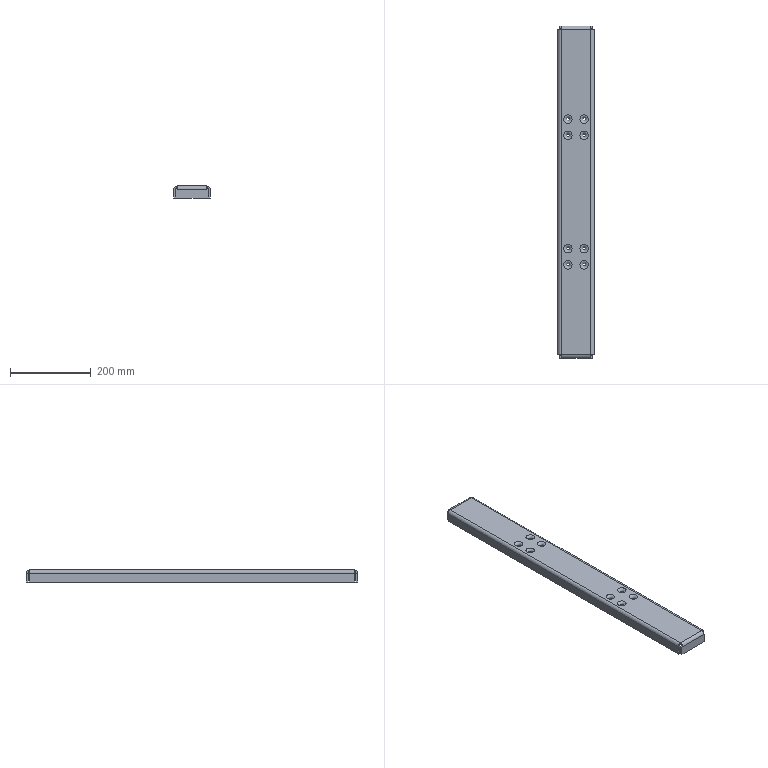Part | NX | features BREP 1 | 1 solid | 78 faces | box 90 x 820 x 30 mm | volume 571533 mm3 | plane 38 | cylinder 24 | torus 16 | commonest cylinder face diameters 6.8 x8 16.8 x8 6 x4 16 x4